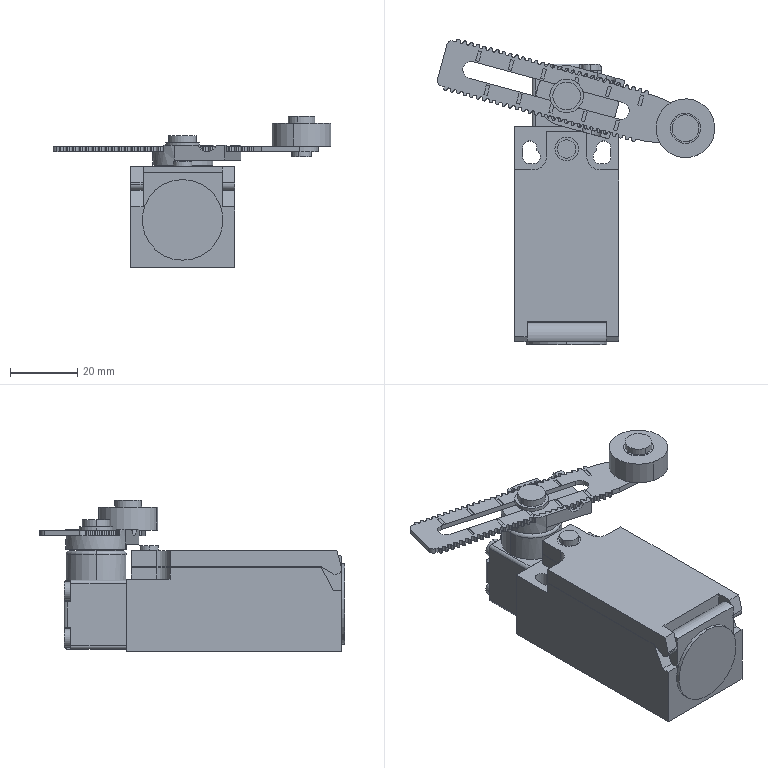Part | SolidWorks | 5 solids | 531 faces | box 82.59 x 90.924 x 45 mm | volume 70601 mm3 | cylinder 341 | plane 188 | torus 2 | commonest cylinder face diameters 1 x237 3 x22 5.5 x10 2 x8 4.3 x7 8 x7